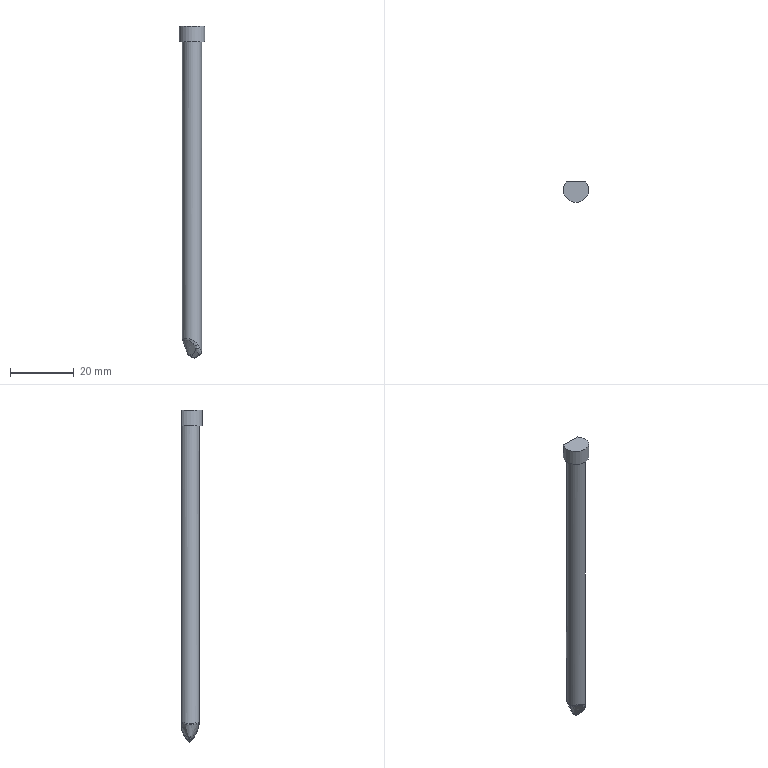Part | 1 solid | 33 faces | box 8 x 6.938 x 104.58 mm | volume 2853 mm3 | spline 15 | plane 6 | cylinder 6 | torus 4 | other 2 | commonest cylinder face diameters 0.7 x2 2.9 x2 6 x1 8 x1